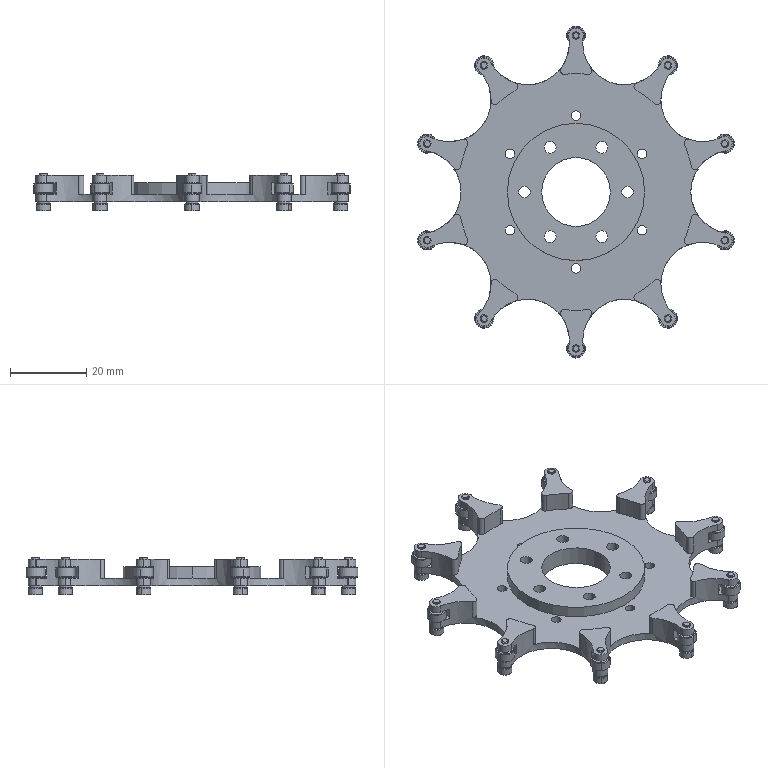Part | SolidWorks | features ReferencePattern 27, LocalCirPattern 1 | 31 solids | 802 faces | box 82.987 x 87 x 9.9 mm | volume 11718 mm3 | cylinder 359 | plane 223 | torus 200 | cone 20 | commonest cylinder face diameters 2 x108 2.7 x40 4.4 x40 3.8 x36 1.6 x20 3.4 x20